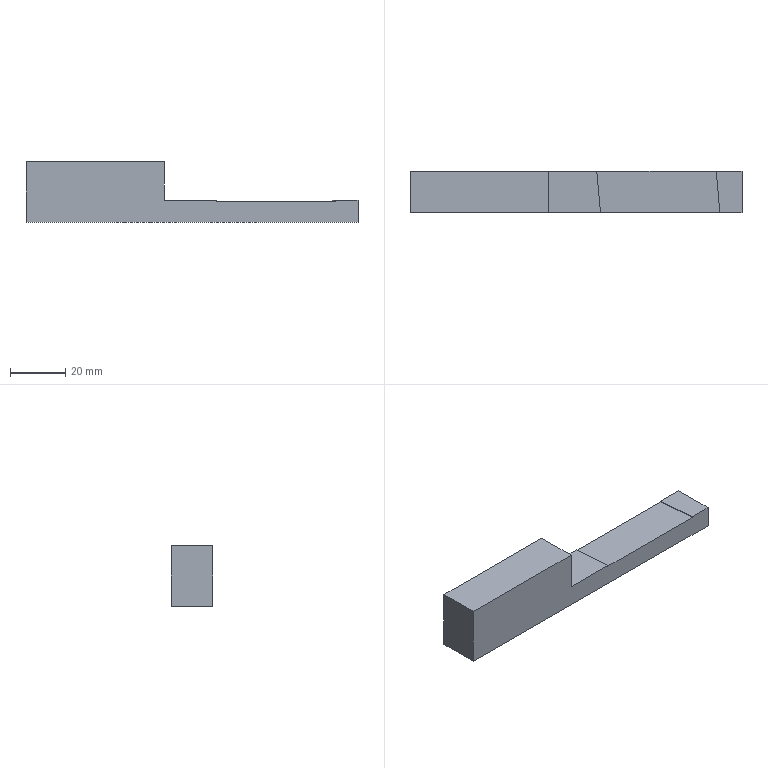Part | SolidWorks | features ICE 4, Extrusion 1 | 1 solid | 12 faces | box 120 x 15 x 22 mm | volume 24706 mm3 | plane 12
STEP:
#1=CARTESIAN_POINT('',(60.,7.5,8.));
#2=VERTEX_POINT('',#1);
#3=CARTESIAN_POINT('',(50.688,7.5,8.));
#4=VERTEX_POINT('',#3);
#5=CARTESIAN_POINT('',(-60.,7.5,8.));
#6=DIRECTION('',(-1.,0.,0.));
#7=VECTOR('',#6,1000.);
#8=LINE('',#5,#7);
#9=EDGE_CURVE('',#2,#4,#8,.T.);
#10=ORIENTED_EDGE('',*,*,#9,.T.);
#11=CARTESIAN_POINT('',(52.,-7.5,8.));
#12=VERTEX_POINT('',#11);
#13=CARTESIAN_POINT('',(50.688,7.5,8.));
#14=DIRECTION('',(-0.08716,0.9962,0.));
#15=VECTOR('',#14,1000.);
#16=LINE('',#13,#15);
#17=EDGE_CURVE('',#12,#4,#16,.T.);
#18=ORIENTED_EDGE('',*,*,#17,.F.);
#19=CARTESIAN_POINT('',(60.,-7.5,8.));
#20=VERTEX_POINT('',#19);
#21=CARTESIAN_POINT('',(-60.,-7.5,8.));
#22=DIRECTION('',(1.,0.,0.));
#23=VECTOR('',#22,1000.);
#24=LINE('',#21,#23);
#25=EDGE_CURVE('',#12,#20,#24,.T.);
#26=ORIENTED_EDGE('',*,*,#25,.T.);
#27=CARTESIAN_POINT('',(60.,-7.5,8.));
#28=DIRECTION('',(0.,1.,0.));
#29=VECTOR('',#28,1000.);
#30=LINE('',#27,#29);
#31=EDGE_CURVE('',#20,#2,#30,.T.);
#32=ORIENTED_EDGE('',*,*,#31,.T.);
#33=EDGE_LOOP('',(#10,#18,#26,#32));
#34=FACE_OUTER_BOUND('',#33,.T.);
#35=CARTESIAN_POINT('',(0.,0.,8.));
#36=DIRECTION('',(0.,0.,-1.));
#37=DIRECTION('',(-1.,0.,0.));
#38=AXIS2_PLACEMENT_3D('',#35,#36,#37);
#39=PLANE('',#38);
#40=ADVANCED_FACE('',(#34),#39,.F.);
#41=CARTESIAN_POINT('',(60.,-7.5,0.));
#42=VERTEX_POINT('',#41);
#43=CARTESIAN_POINT('',(60.,7.5,0.));
#44=VERTEX_POINT('',#43);
#45=CARTESIAN_POINT('',(60.,-7.5,0.));
#46=DIRECTION('',(0.,1.,0.));
#47=VECTOR('',#46,1000.);
#48=LINE('',#45,#47);
#49=EDGE_CURVE('',#42,#44,#48,.T.);
#50=ORIENTED_EDGE('',*,*,#49,.T.);
#51=CARTESIAN_POINT('',(60.,7.5,8.));
#52=DIRECTION('',(0.,0.,-1.));
#53=VECTOR('',#52,1000.);
#54=LINE('',#51,#53);
#55=EDGE_CURVE('',#2,#44,#54,.T.);
#56=ORIENTED_EDGE('',*,*,#55,.F.);
#57=ORIENTED_EDGE('',*,*,#31,.F.);
#58=CARTESIAN_POINT('',(60.,-7.5,8.));
#59=DIRECTION('',(0.,0.,-1.));
#60=VECTOR('',#59,1000.);
#61=LINE('',#58,#60);
#62=EDGE_CURVE('',#20,#42,#61,.T.);
#63=ORIENTED_EDGE('',*,*,#62,.T.);
#64=EDGE_LOOP('',(#50,#56,#57,#63));
#65=FACE_OUTER_BOUND('',#64,.T.);
#66=CARTESIAN_POINT('',(60.,-7.5,8.));
#67=DIRECTION('',(-1.,0.,0.));
#68=DIRECTION('',(0.,0.,1.));
#69=AXIS2_PLACEMENT_3D('',#66,#67,#68);
#70=PLANE('',#69);
#71=ADVANCED_FACE('',(#65),#70,.F.);
#72=CARTESIAN_POINT('',(50.688,7.5,7.7));
#73=VERTEX_POINT('',#72);
#74=CARTESIAN_POINT('',(7.523,7.5,7.7));
#75=VERTEX_POINT('',#74);
#76=CARTESIAN_POINT('',(7.523,7.5,7.7));
#77=DIRECTION('',(-1.,0.,0.));
#78=VECTOR('',#77,1000.);
#79=LINE('',#76,#78);
#80=EDGE_CURVE('',#73,#75,#79,.T.);
#81=ORIENTED_EDGE('',*,*,#80,.F.);
#82=CARTESIAN_POINT('',(50.688,7.5,7.7));
#83=DIRECTION('',(0.,0.,1.));
#84=VECTOR('',#83,1000.);
#85=LINE('',#82,#84);
#86=EDGE_CURVE('',#73,#4,#85,.T.);
#87=ORIENTED_EDGE('',*,*,#86,.T.);
#88=ORIENTED_EDGE('',*,*,#9,.F.);
#89=ORIENTED_EDGE('',*,*,#55,.T.);
#90=CARTESIAN_POINT('',(-60.,7.5,0.));
#91=VERTEX_POINT('',#90);
#92=CARTESIAN_POINT('',(-60.,7.5,0.));
#93=DIRECTION('',(-1.,0.,0.));
#94=VECTOR('',#93,1000.);
#95=LINE('',#92,#94);
#96=EDGE_CURVE('',#44,#91,#95,.T.);
#97=ORIENTED_EDGE('',*,*,#96,.T.);
#98=CARTESIAN_POINT('',(-60.,7.5,22.));
#99=VERTEX_POINT('',#98);
#100=CARTESIAN_POINT('',(-60.,7.5,8.));
#101=DIRECTION('',(0.,0.,-1.));
#102=VECTOR('',#101,1000.);
#103=LINE('',#100,#102);
#104=EDGE_CURVE('',#99,#91,#103,.T.);
#105=ORIENTED_EDGE('',*,*,#104,.F.);
#106=CARTESIAN_POINT('',(-10.,7.5,22.));
#107=VERTEX_POINT('',#106);
#108=CARTESIAN_POINT('',(-60.,7.5,22.));
#109=DIRECTION('',(1.,0.,0.));
#110=VECTOR('',#109,1000.);
#111=LINE('',#108,#110);
#112=EDGE_CURVE('',#99,#107,#111,.T.);
#113=ORIENTED_EDGE('',*,*,#112,.T.);
#114=CARTESIAN_POINT('',(-10.,7.5,8.));
#115=VERTEX_POINT('',#114);
#116=CARTESIAN_POINT('',(-10.,7.5,8.));
#117=DIRECTION('',(0.,0.,-1.));
#118=VECTOR('',#117,1000.);
#119=LINE('',#116,#118);
#120=EDGE_CURVE('',#107,#115,#119,.T.);
#121=ORIENTED_EDGE('',*,*,#120,.T.);
#122=CARTESIAN_POINT('',(7.523,7.5,8.));
#123=VERTEX_POINT('',#122);
#124=CARTESIAN_POINT('',(-60.,7.5,8.));
#125=DIRECTION('',(-1.,0.,0.));
#126=VECTOR('',#125,1000.);
#127=LINE('',#124,#126);
#128=EDGE_CURVE('',#123,#115,#127,.T.);
#129=ORIENTED_EDGE('',*,*,#128,.F.);
#130=CARTESIAN_POINT('',(7.523,7.5,7.7));
#131=DIRECTION('',(0.,0.,1.));
#132=VECTOR('',#131,1000.);
#133=LINE('',#130,#132);
#134=EDGE_CURVE('',#75,#123,#133,.T.);
#135=ORIENTED_EDGE('',*,*,#134,.F.);
#136=EDGE_LOOP('',(#81,#87,#88,#89,#97,#105,#113,#121,#129,#135));
#137=FACE_OUTER_BOUND('',#136,.T.);
#138=CARTESIAN_POINT('',(-60.,7.5,8.));
#139=DIRECTION('',(0.,-1.,0.));
#140=DIRECTION('',(0.,0.,-1.));
#141=AXIS2_PLACEMENT_3D('',#138,#139,#140);
#142=PLANE('',#141);
#143=ADVANCED_FACE('',(#137),#142,.F.);
#144=CARTESIAN_POINT('',(-60.,-7.5,0.));
#145=VERTEX_POINT('',#144);
#146=CARTESIAN_POINT('',(-60.,-7.5,0.));
#147=DIRECTION('',(0.,-1.,0.));
#148=VECTOR('',#147,1000.);
#149=LINE('',#146,#148);
#150=EDGE_CURVE('',#91,#145,#149,.T.);
#151=ORIENTED_EDGE('',*,*,#150,.T.);
#152=CARTESIAN_POINT('',(-60.,-7.5,22.));
#153=VERTEX_POINT('',#152);
#154=CARTESIAN_POINT('',(-60.,-7.5,8.));
#155=DIRECTION('',(0.,0.,-1.));
#156=VECTOR('',#155,1000.);
#157=LINE('',#154,#156);
#158=EDGE_CURVE('',#153,#145,#157,.T.);
#159=ORIENTED_EDGE('',*,*,#158,.F.);
#160=CARTESIAN_POINT('',(-60.,59.423,22.));
#161=DIRECTION('',(0.,-1.,0.));
#162=VECTOR('',#161,1000.);
#163=LINE('',#160,#162);
#164=EDGE_CURVE('',#99,#153,#163,.T.);
#165=ORIENTED_EDGE('',*,*,#164,.F.);
#166=ORIENTED_EDGE('',*,*,#104,.T.);
#167=EDGE_LOOP('',(#151,#159,#165,#166));
#168=FACE_OUTER_BOUND('',#167,.T.);
#169=CARTESIAN_POINT('',(-60.,-7.5,8.));
#170=DIRECTION('',(1.,0.,0.));
#171=DIRECTION('',(0.,0.,-1.));
#172=AXIS2_PLACEMENT_3D('',#169,#170,#171);
#173=PLANE('',#172);
#174=ADVANCED_FACE('',(#168),#173,.F.);
#175=ORIENTED_EDGE('',*,*,#25,.F.);
#176=CARTESIAN_POINT('',(52.,-7.5,7.7));
#177=VERTEX_POINT('',#176);
#178=CARTESIAN_POINT('',(52.,-7.5,7.7));
#179=DIRECTION('',(0.,0.,1.));
#180=VECTOR('',#179,1000.);
#181=LINE('',#178,#180);
#182=EDGE_CURVE('',#177,#12,#181,.T.);
#183=ORIENTED_EDGE('',*,*,#182,.F.);
#184=CARTESIAN_POINT('',(8.836,-7.5,7.7));
#185=VERTEX_POINT('',#184);
#186=CARTESIAN_POINT('',(8.836,-7.5,7.7));
#187=DIRECTION('',(1.,0.,0.));
#188=VECTOR('',#187,1000.);
#189=LINE('',#186,#188);
#190=EDGE_CURVE('',#185,#177,#189,.T.);
#191=ORIENTED_EDGE('',*,*,#190,.F.);
#192=CARTESIAN_POINT('',(8.836,-7.5,8.));
#193=VERTEX_POINT('',#192);
#194=CARTESIAN_POINT('',(8.836,-7.5,7.7));
#195=DIRECTION('',(0.,0.,1.));
#196=VECTOR('',#195,1000.);
#197=LINE('',#194,#196);
#198=EDGE_CURVE('',#185,#193,#197,.T.);
#199=ORIENTED_EDGE('',*,*,#198,.T.);
#200=CARTESIAN_POINT('',(-10.,-7.5,8.));
#201=VERTEX_POINT('',#200);
#202=CARTESIAN_POINT('',(-60.,-7.5,8.));
#203=DIRECTION('',(1.,0.,0.));
#204=VECTOR('',#203,1000.);
#205=LINE('',#202,#204);
#206=EDGE_CURVE('',#201,#193,#205,.T.);
#207=ORIENTED_EDGE('',*,*,#206,.F.);
#208=CARTESIAN_POINT('',(-10.,-7.5,22.));
#209=VERTEX_POINT('',#208);
#210=CARTESIAN_POINT('',(-10.,-7.5,8.));
#211=DIRECTION('',(0.,0.,1.));
#212=VECTOR('',#211,1000.);
#213=LINE('',#210,#212);
#214=EDGE_CURVE('',#201,#209,#213,.T.);
#215=ORIENTED_EDGE('',*,*,#214,.T.);
#216=CARTESIAN_POINT('',(-60.,-7.5,22.));
#217=DIRECTION('',(-1.,0.,0.));
#218=VECTOR('',#217,1000.);
#219=LINE('',#216,#218);
#220=EDGE_CURVE('',#209,#153,#219,.T.);
#221=ORIENTED_EDGE('',*,*,#220,.T.);
#222=ORIENTED_EDGE('',*,*,#158,.T.);
#223=CARTESIAN_POINT('',(-60.,-7.5,0.));
#224=DIRECTION('',(1.,0.,0.));
#225=VECTOR('',#224,1000.);
#226=LINE('',#223,#225);
#227=EDGE_CURVE('',#145,#42,#226,.T.);
#228=ORIENTED_EDGE('',*,*,#227,.T.);
#229=ORIENTED_EDGE('',*,*,#62,.F.);
#230=EDGE_LOOP('',(#175,#183,#191,#199,#207,#215,#221,#222,#228,#229));
#231=FACE_OUTER_BOUND('',#230,.T.);
#232=CARTESIAN_POINT('',(-60.,-7.5,8.));
#233=DIRECTION('',(0.,1.,0.));
#234=DIRECTION('',(0.,0.,1.));
#235=AXIS2_PLACEMENT_3D('',#232,#233,#234);
#236=PLANE('',#235);
#237=ADVANCED_FACE('',(#231),#236,.F.);
#238=ORIENTED_EDGE('',*,*,#128,.T.);
#239=CARTESIAN_POINT('',(-10.,59.423,8.));
#240=DIRECTION('',(0.,-1.,0.));
#241=VECTOR('',#240,1000.);
#242=LINE('',#239,#241);
#243=EDGE_CURVE('',#115,#201,#242,.T.);
#244=ORIENTED_EDGE('',*,*,#243,.T.);
#245=ORIENTED_EDGE('',*,*,#206,.T.);
#246=CARTESIAN_POINT('',(7.523,7.5,8.));
#247=DIRECTION('',(0.08716,-0.9962,0.));
#248=VECTOR('',#247,1000.);
#249=LINE('',#246,#248);
#250=EDGE_CURVE('',#123,#193,#249,.T.);
#251=ORIENTED_EDGE('',*,*,#250,.F.);
#252=EDGE_LOOP('',(#238,#244,#245,#251));
#253=FACE_OUTER_BOUND('',#252,.T.);
#254=CARTESIAN_POINT('',(0.,0.,8.));
#255=DIRECTION('',(0.,0.,-1.));
#256=DIRECTION('',(-1.,0.,0.));
#257=AXIS2_PLACEMENT_3D('',#254,#255,#256);
#258=PLANE('',#257);
#259=ADVANCED_FACE('',(#253),#258,.F.);
#260=ORIENTED_EDGE('',*,*,#49,.F.);
#261=ORIENTED_EDGE('',*,*,#227,.F.);
#262=ORIENTED_EDGE('',*,*,#150,.F.);
#263=ORIENTED_EDGE('',*,*,#96,.F.);
#264=EDGE_LOOP('',(#260,#261,#262,#263));
#265=FACE_OUTER_BOUND('',#264,.T.);
#266=CARTESIAN_POINT('',(0.,0.,0.));
#267=DIRECTION('',(0.,0.,-1.));
#268=DIRECTION('',(-1.,0.,0.));
#269=AXIS2_PLACEMENT_3D('',#266,#267,#268);
#270=PLANE('',#269);
#271=ADVANCED_FACE('',(#265),#270,.T.);
#272=ORIENTED_EDGE('',*,*,#17,.T.);
#273=ORIENTED_EDGE('',*,*,#86,.F.);
#274=CARTESIAN_POINT('',(50.688,7.5,7.7));
#275=DIRECTION('',(-0.08716,0.9962,0.));
#276=VECTOR('',#275,1000.);
#277=LINE('',#274,#276);
#278=EDGE_CURVE('',#177,#73,#277,.T.);
#279=ORIENTED_EDGE('',*,*,#278,.F.);
#280=ORIENTED_EDGE('',*,*,#182,.T.);
#281=EDGE_LOOP('',(#272,#273,#279,#280));
#282=FACE_OUTER_BOUND('',#281,.T.);
#283=CARTESIAN_POINT('',(50.688,7.5,7.7));
#284=DIRECTION('',(0.9962,0.08716,0.));
#285=DIRECTION('',(-0.08716,0.9962,0.));
#286=AXIS2_PLACEMENT_3D('',#283,#284,#285);
#287=PLANE('',#286);
#288=ADVANCED_FACE('',(#282),#287,.F.);
#289=ORIENTED_EDGE('',*,*,#250,.T.);
#290=ORIENTED_EDGE('',*,*,#198,.F.);
#291=CARTESIAN_POINT('',(7.523,7.5,7.7));
#292=DIRECTION('',(0.08716,-0.9962,0.));
#293=VECTOR('',#292,1000.);
#294=LINE('',#291,#293);
#295=EDGE_CURVE('',#75,#185,#294,.T.);
#296=ORIENTED_EDGE('',*,*,#295,.F.);
#297=ORIENTED_EDGE('',*,*,#134,.T.);
#298=EDGE_LOOP('',(#289,#290,#296,#297));
#299=FACE_OUTER_BOUND('',#298,.T.);
#300=CARTESIAN_POINT('',(7.523,7.5,7.7));
#301=DIRECTION('',(-0.9962,-0.08716,0.));
#302=DIRECTION('',(0.08716,-0.9962,0.));
#303=AXIS2_PLACEMENT_3D('',#300,#301,#302);
#304=PLANE('',#303);
#305=ADVANCED_FACE('',(#299),#304,.F.);
#306=ORIENTED_EDGE('',*,*,#80,.T.);
#307=ORIENTED_EDGE('',*,*,#295,.T.);
#308=ORIENTED_EDGE('',*,*,#190,.T.);
#309=ORIENTED_EDGE('',*,*,#278,.T.);
#310=EDGE_LOOP('',(#306,#307,#308,#309));
#311=FACE_OUTER_BOUND('',#310,.T.);
#312=CARTESIAN_POINT('',(0.,0.,7.7));
#313=DIRECTION('',(0.,0.,-1.));
#314=DIRECTION('',(-1.,0.,0.));
#315=AXIS2_PLACEMENT_3D('',#312,#313,#314);
#316=PLANE('',#315);
#317=ADVANCED_FACE('',(#311),#316,.F.);
#318=ORIENTED_EDGE('',*,*,#112,.F.);
#319=ORIENTED_EDGE('',*,*,#164,.T.);
#320=ORIENTED_EDGE('',*,*,#220,.F.);
#321=CARTESIAN_POINT('',(-10.,59.423,22.));
#322=DIRECTION('',(0.,-1.,0.));
#323=VECTOR('',#322,1000.);
#324=LINE('',#321,#323);
#325=EDGE_CURVE('',#107,#209,#324,.T.);
#326=ORIENTED_EDGE('',*,*,#325,.F.);
#327=EDGE_LOOP('',(#318,#319,#320,#326));
#328=FACE_OUTER_BOUND('',#327,.T.);
#329=CARTESIAN_POINT('',(-60.,59.423,22.));
#330=DIRECTION('',(0.,0.,1.));
#331=DIRECTION('',(1.,0.,0.));
#332=AXIS2_PLACEMENT_3D('',#329,#330,#331);
#333=PLANE('',#332);
#334=ADVANCED_FACE('',(#328),#333,.T.);
#335=ORIENTED_EDGE('',*,*,#120,.F.);
#336=ORIENTED_EDGE('',*,*,#325,.T.);
#337=ORIENTED_EDGE('',*,*,#214,.F.);
#338=ORIENTED_EDGE('',*,*,#243,.F.);
#339=EDGE_LOOP('',(#335,#336,#337,#338));
#340=FACE_OUTER_BOUND('',#339,.T.);
#341=CARTESIAN_POINT('',(-10.,59.423,8.));
#342=DIRECTION('',(1.,0.,0.));
#343=DIRECTION('',(0.,0.,-1.));
#344=AXIS2_PLACEMENT_3D('',#341,#342,#343);
#345=PLANE('',#344);
#346=ADVANCED_FACE('',(#340),#345,.T.);
#347=CLOSED_SHELL('',(#40,#71,#143,#174,#237,#259,#271,#288,#305,#317,#334,#346));
#348=MANIFOLD_SOLID_BREP('',#347);
#349=CARTESIAN_POINT('',(0.,0.,0.));
#350=DIRECTION('',(0.,0.,1.));
#351=DIRECTION('',(1.,0.,0.));
#352=AXIS2_PLACEMENT_3D('',#349,#350,#351);
#353=(LENGTH_UNIT()NAMED_UNIT(*)SI_UNIT(.MILLI.,.METRE.));
#354=UNCERTAINTY_MEASURE_WITH_UNIT(LENGTH_MEASURE(0.00001),#353,'','');
#355=(NAMED_UNIT(*)PLANE_ANGLE_UNIT()SI_UNIT($,.RADIAN.));
#356=(NAMED_UNIT(*)SI_UNIT($,.STERADIAN.)SOLID_ANGLE_UNIT());
#357=(GEOMETRIC_REPRESENTATION_CONTEXT(3)GLOBAL_UNCERTAINTY_ASSIGNED_CONTEXT((#354))GLOBAL_UNIT_ASSIGNED_CONTEXT((#353,#355,#356))REPRESENTATION_CONTEXT('',''));
#358=ADVANCED_BREP_SHAPE_REPRESENTATION('',(#348,#352),#357);